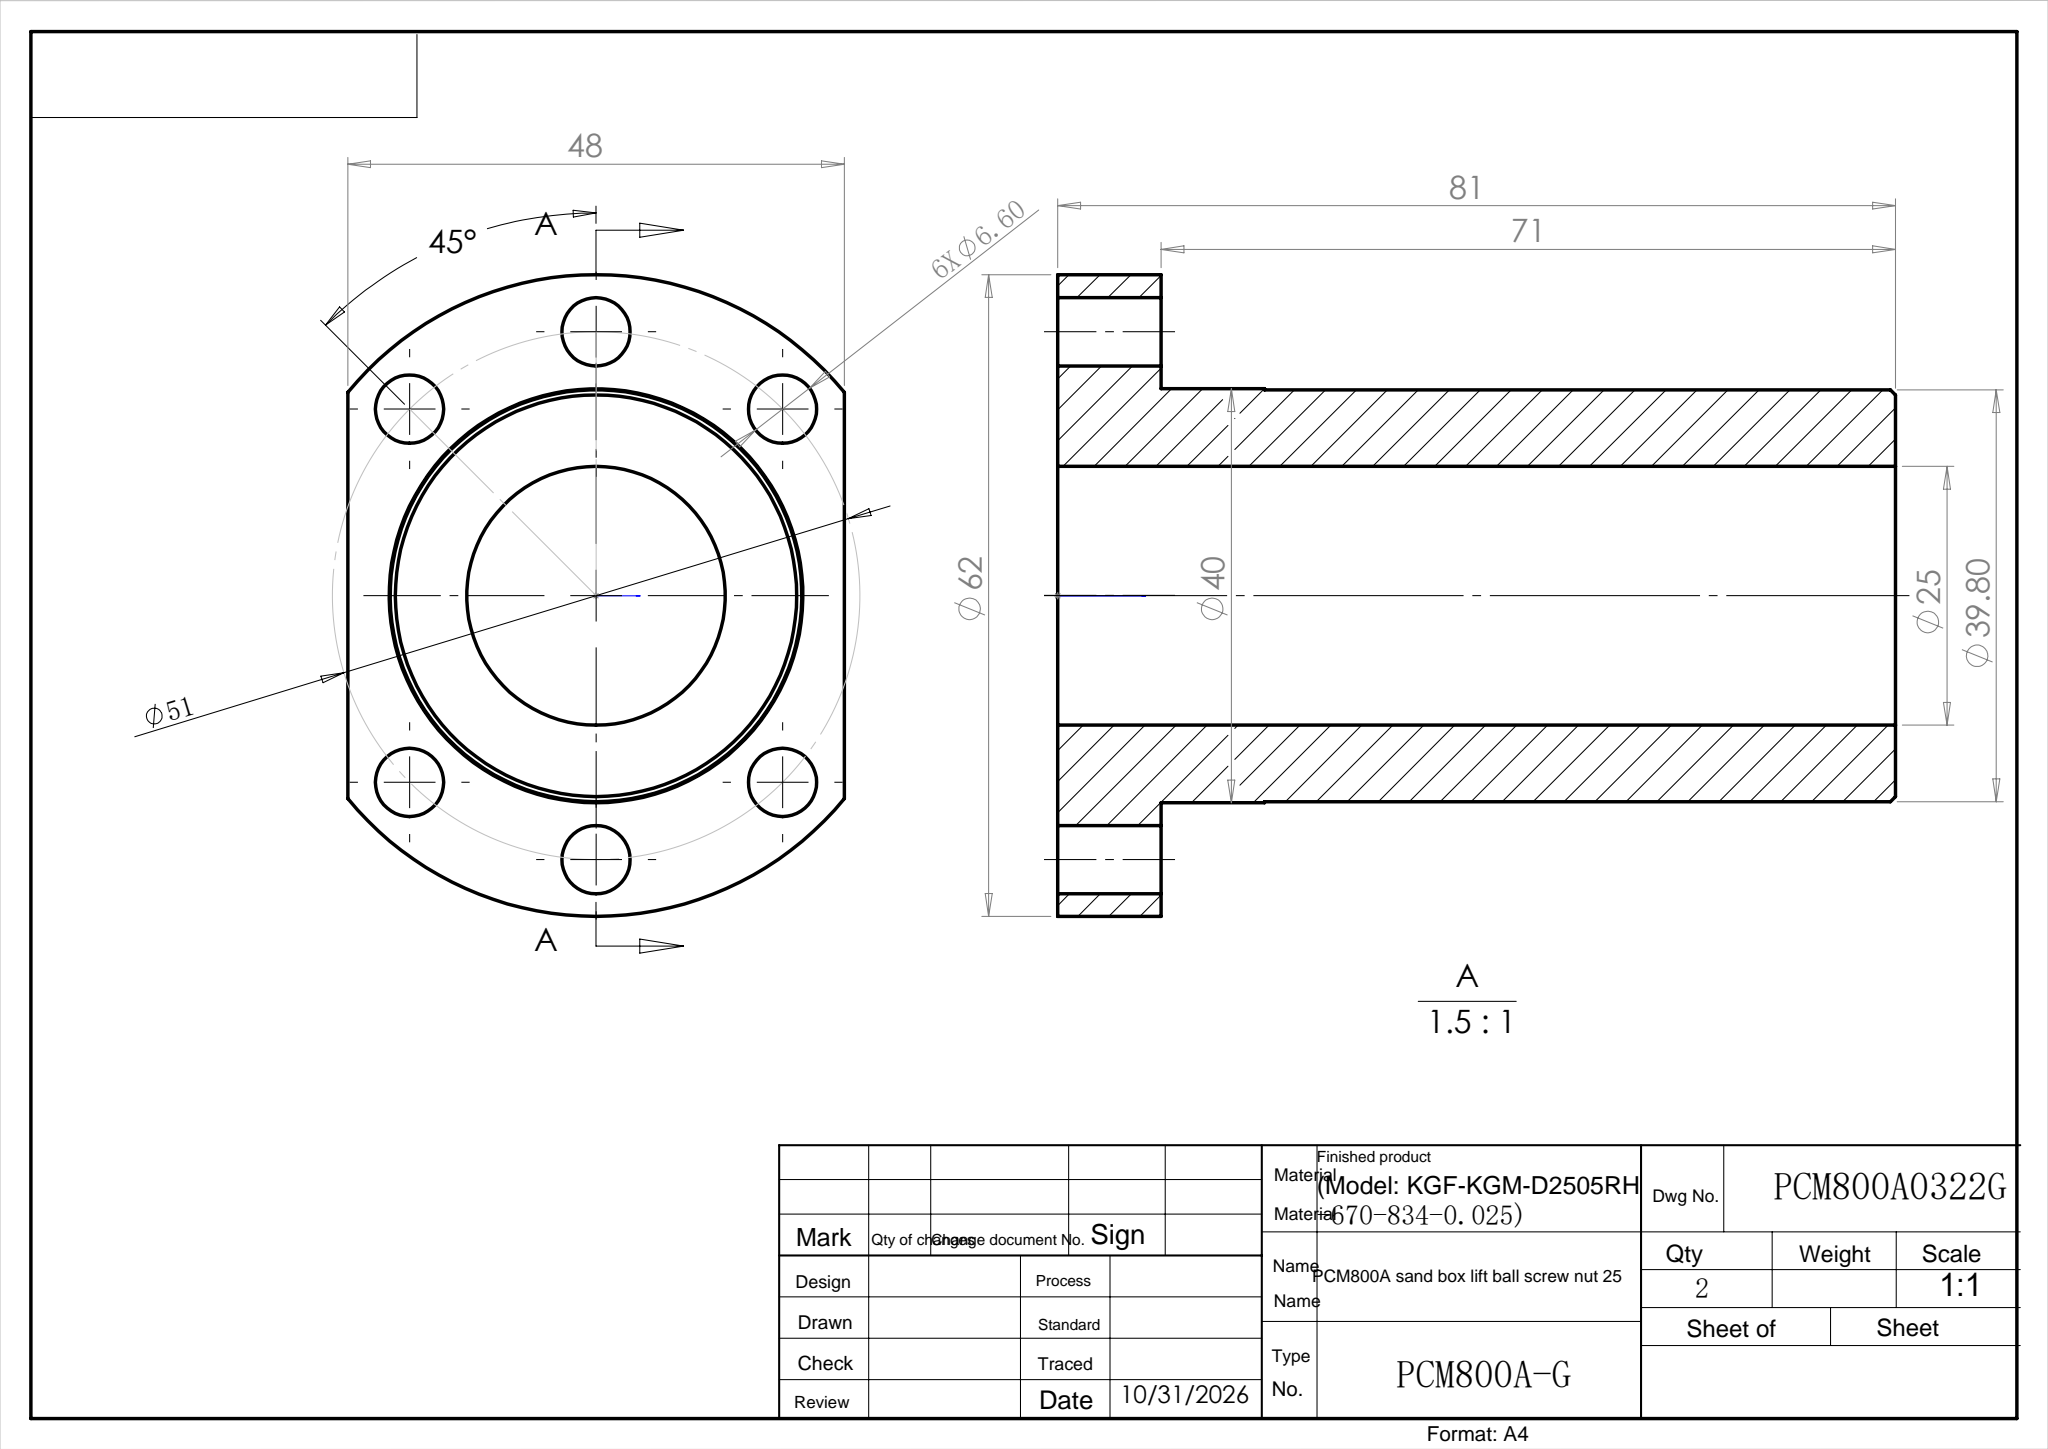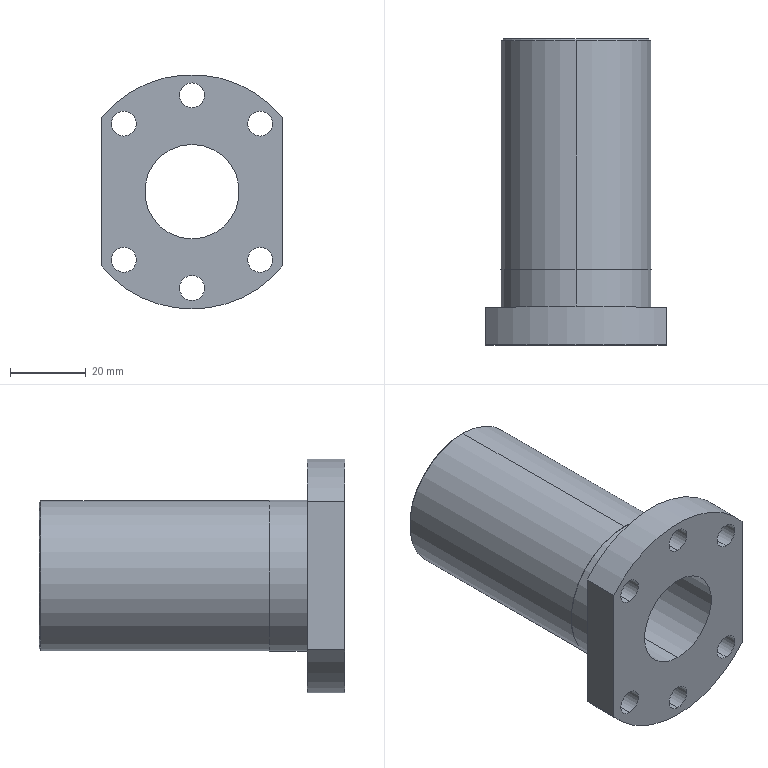Part | SolidWorks | features Boss 2, Cut 2, Chamfer 1, Extrusion 1 | 1 solid | 29 faces | box 48 x 81 x 62 mm | volume 73064 mm3 | cylinder 21 | plane 6 | cone 2 | commonest cylinder face diameters 6.6 x12 62 x3 25 x2 39.8 x2 40 x2
STEP:
#1=CARTESIAN_POINT('',(0.,81.,19.4));
#2=VERTEX_POINT('',#1);
#3=CARTESIAN_POINT('',(0.,81.,-19.4));
#4=VERTEX_POINT('',#3);
#5=CARTESIAN_POINT('',(0.,81.,0.));
#6=DIRECTION('',(0.,1.,0.));
#7=DIRECTION('',(0.,0.,1.));
#8=AXIS2_PLACEMENT_3D('',#5,#6,#7);
#9=CIRCLE('',#8,19.4);
#10=EDGE_CURVE('',#2,#4,#9,.T.);
#11=ORIENTED_EDGE('',*,*,#10,.F.);
#12=CARTESIAN_POINT('',(0.,80.5,19.9));
#13=VERTEX_POINT('',#12);
#14=CARTESIAN_POINT('',(0.,81.,19.4));
#15=DIRECTION('',(0.,-0.7071,0.7071));
#16=VECTOR('',#15,1000.);
#17=LINE('',#14,#16);
#18=EDGE_CURVE('',#2,#13,#17,.T.);
#19=ORIENTED_EDGE('',*,*,#18,.T.);
#20=CARTESIAN_POINT('',(0.,80.5,-19.9));
#21=VERTEX_POINT('',#20);
#22=CARTESIAN_POINT('',(0.,80.5,0.));
#23=DIRECTION('',(0.,-1.,0.));
#24=DIRECTION('',(0.,0.,1.));
#25=AXIS2_PLACEMENT_3D('',#22,#23,#24);
#26=CIRCLE('',#25,19.9);
#27=EDGE_CURVE('',#21,#13,#26,.T.);
#28=ORIENTED_EDGE('',*,*,#27,.F.);
#29=CARTESIAN_POINT('',(0.,81.,-19.4));
#30=DIRECTION('',(0.,-0.7071,-0.7071));
#31=VECTOR('',#30,1000.);
#32=LINE('',#29,#31);
#33=EDGE_CURVE('',#4,#21,#32,.T.);
#34=ORIENTED_EDGE('',*,*,#33,.F.);
#35=EDGE_LOOP('',(#11,#19,#28,#34));
#36=FACE_OUTER_BOUND('',#35,.T.);
#37=CARTESIAN_POINT('',(0.,81.,0.));
#38=DIRECTION('',(0.,-1.,0.));
#39=DIRECTION('',(0.,0.,-1.));
#40=AXIS2_PLACEMENT_3D('',#37,#38,#39);
#41=CONICAL_SURFACE('',#40,19.4,0.7854);
#42=ADVANCED_FACE('',(#36),#41,.T.);
#43=CARTESIAN_POINT('',(18.031,10.,14.731));
#44=VERTEX_POINT('',#43);
#45=CARTESIAN_POINT('',(18.031,10.,21.331));
#46=VERTEX_POINT('',#45);
#47=CARTESIAN_POINT('',(18.031,10.,18.031));
#48=DIRECTION('',(0.,1.,0.));
#49=DIRECTION('',(0.,0.,1.));
#50=AXIS2_PLACEMENT_3D('',#47,#48,#49);
#51=CIRCLE('',#50,3.3);
#52=EDGE_CURVE('',#44,#46,#51,.T.);
#53=ORIENTED_EDGE('',*,*,#52,.T.);
#54=CARTESIAN_POINT('',(18.031,0.,21.331));
#55=VERTEX_POINT('',#54);
#56=CARTESIAN_POINT('',(18.031,81.,21.331));
#57=DIRECTION('',(0.,-1.,0.));
#58=VECTOR('',#57,1000.);
#59=LINE('',#56,#58);
#60=EDGE_CURVE('',#46,#55,#59,.T.);
#61=ORIENTED_EDGE('',*,*,#60,.T.);
#62=CARTESIAN_POINT('',(18.031,0.,14.731));
#63=VERTEX_POINT('',#62);
#64=CARTESIAN_POINT('',(18.031,0.,18.031));
#65=DIRECTION('',(0.,-1.,0.));
#66=DIRECTION('',(0.,0.,-1.));
#67=AXIS2_PLACEMENT_3D('',#64,#65,#66);
#68=CIRCLE('',#67,3.3);
#69=EDGE_CURVE('',#55,#63,#68,.T.);
#70=ORIENTED_EDGE('',*,*,#69,.T.);
#71=CARTESIAN_POINT('',(18.031,81.,14.731));
#72=DIRECTION('',(0.,-1.,0.));
#73=VECTOR('',#72,1000.);
#74=LINE('',#71,#73);
#75=EDGE_CURVE('',#44,#63,#74,.T.);
#76=ORIENTED_EDGE('',*,*,#75,.F.);
#77=EDGE_LOOP('',(#53,#61,#70,#76));
#78=FACE_OUTER_BOUND('',#77,.T.);
#79=CARTESIAN_POINT('',(18.031,81.,18.031));
#80=DIRECTION('',(0.,-1.,0.));
#81=DIRECTION('',(0.,0.,-1.));
#82=AXIS2_PLACEMENT_3D('',#79,#80,#81);
#83=CYLINDRICAL_SURFACE('',#82,3.3);
#84=ADVANCED_FACE('',(#78),#83,.F.);
#85=CARTESIAN_POINT('',(0.,10.,22.2));
#86=VERTEX_POINT('',#85);
#87=CARTESIAN_POINT('',(0.,10.,28.8));
#88=VERTEX_POINT('',#87);
#89=CARTESIAN_POINT('',(0.,10.,25.5));
#90=DIRECTION('',(0.,1.,0.));
#91=DIRECTION('',(0.,0.,1.));
#92=AXIS2_PLACEMENT_3D('',#89,#90,#91);
#93=CIRCLE('',#92,3.3);
#94=EDGE_CURVE('',#86,#88,#93,.T.);
#95=ORIENTED_EDGE('',*,*,#94,.T.);
#96=CARTESIAN_POINT('',(0.,0.,28.8));
#97=VERTEX_POINT('',#96);
#98=CARTESIAN_POINT('',(0.,81.,28.8));
#99=DIRECTION('',(0.,-1.,0.));
#100=VECTOR('',#99,1000.);
#101=LINE('',#98,#100);
#102=EDGE_CURVE('',#88,#97,#101,.T.);
#103=ORIENTED_EDGE('',*,*,#102,.T.);
#104=CARTESIAN_POINT('',(0.,0.,22.2));
#105=VERTEX_POINT('',#104);
#106=CARTESIAN_POINT('',(0.,0.,25.5));
#107=DIRECTION('',(0.,-1.,0.));
#108=DIRECTION('',(0.,0.,-1.));
#109=AXIS2_PLACEMENT_3D('',#106,#107,#108);
#110=CIRCLE('',#109,3.3);
#111=EDGE_CURVE('',#97,#105,#110,.T.);
#112=ORIENTED_EDGE('',*,*,#111,.T.);
#113=CARTESIAN_POINT('',(0.,81.,22.2));
#114=DIRECTION('',(0.,-1.,0.));
#115=VECTOR('',#114,1000.);
#116=LINE('',#113,#115);
#117=EDGE_CURVE('',#86,#105,#116,.T.);
#118=ORIENTED_EDGE('',*,*,#117,.F.);
#119=EDGE_LOOP('',(#95,#103,#112,#118));
#120=FACE_OUTER_BOUND('',#119,.T.);
#121=CARTESIAN_POINT('',(0.,81.,25.5));
#122=DIRECTION('',(0.,-1.,0.));
#123=DIRECTION('',(0.,0.,-1.));
#124=AXIS2_PLACEMENT_3D('',#121,#122,#123);
#125=CYLINDRICAL_SURFACE('',#124,3.3);
#126=ADVANCED_FACE('',(#120),#125,.F.);
#127=CARTESIAN_POINT('',(-18.031,10.,14.731));
#128=VERTEX_POINT('',#127);
#129=CARTESIAN_POINT('',(-18.031,10.,21.331));
#130=VERTEX_POINT('',#129);
#131=CARTESIAN_POINT('',(-18.031,10.,18.031));
#132=DIRECTION('',(0.,1.,0.));
#133=DIRECTION('',(0.,0.,1.));
#134=AXIS2_PLACEMENT_3D('',#131,#132,#133);
#135=CIRCLE('',#134,3.3);
#136=EDGE_CURVE('',#128,#130,#135,.T.);
#137=ORIENTED_EDGE('',*,*,#136,.T.);
#138=CARTESIAN_POINT('',(-18.031,0.,21.331));
#139=VERTEX_POINT('',#138);
#140=CARTESIAN_POINT('',(-18.031,81.,21.331));
#141=DIRECTION('',(0.,-1.,0.));
#142=VECTOR('',#141,1000.);
#143=LINE('',#140,#142);
#144=EDGE_CURVE('',#130,#139,#143,.T.);
#145=ORIENTED_EDGE('',*,*,#144,.T.);
#146=CARTESIAN_POINT('',(-18.031,0.,14.731));
#147=VERTEX_POINT('',#146);
#148=CARTESIAN_POINT('',(-18.031,0.,18.031));
#149=DIRECTION('',(0.,-1.,0.));
#150=DIRECTION('',(0.,0.,-1.));
#151=AXIS2_PLACEMENT_3D('',#148,#149,#150);
#152=CIRCLE('',#151,3.3);
#153=EDGE_CURVE('',#139,#147,#152,.T.);
#154=ORIENTED_EDGE('',*,*,#153,.T.);
#155=CARTESIAN_POINT('',(-18.031,81.,14.731));
#156=DIRECTION('',(0.,-1.,0.));
#157=VECTOR('',#156,1000.);
#158=LINE('',#155,#157);
#159=EDGE_CURVE('',#128,#147,#158,.T.);
#160=ORIENTED_EDGE('',*,*,#159,.F.);
#161=EDGE_LOOP('',(#137,#145,#154,#160));
#162=FACE_OUTER_BOUND('',#161,.T.);
#163=CARTESIAN_POINT('',(-18.031,81.,18.031));
#164=DIRECTION('',(0.,-1.,0.));
#165=DIRECTION('',(0.,0.,-1.));
#166=AXIS2_PLACEMENT_3D('',#163,#164,#165);
#167=CYLINDRICAL_SURFACE('',#166,3.3);
#168=ADVANCED_FACE('',(#162),#167,.F.);
#169=CARTESIAN_POINT('',(-18.031,10.,-21.331));
#170=VERTEX_POINT('',#169);
#171=CARTESIAN_POINT('',(-18.031,10.,-14.731));
#172=VERTEX_POINT('',#171);
#173=CARTESIAN_POINT('',(-18.031,10.,-18.031));
#174=DIRECTION('',(0.,1.,0.));
#175=DIRECTION('',(0.,0.,1.));
#176=AXIS2_PLACEMENT_3D('',#173,#174,#175);
#177=CIRCLE('',#176,3.3);
#178=EDGE_CURVE('',#170,#172,#177,.T.);
#179=ORIENTED_EDGE('',*,*,#178,.T.);
#180=CARTESIAN_POINT('',(-18.031,0.,-14.731));
#181=VERTEX_POINT('',#180);
#182=CARTESIAN_POINT('',(-18.031,81.,-14.731));
#183=DIRECTION('',(0.,-1.,0.));
#184=VECTOR('',#183,1000.);
#185=LINE('',#182,#184);
#186=EDGE_CURVE('',#172,#181,#185,.T.);
#187=ORIENTED_EDGE('',*,*,#186,.T.);
#188=CARTESIAN_POINT('',(-18.031,0.,-21.331));
#189=VERTEX_POINT('',#188);
#190=CARTESIAN_POINT('',(-18.031,0.,-18.031));
#191=DIRECTION('',(0.,-1.,0.));
#192=DIRECTION('',(0.,0.,-1.));
#193=AXIS2_PLACEMENT_3D('',#190,#191,#192);
#194=CIRCLE('',#193,3.3);
#195=EDGE_CURVE('',#181,#189,#194,.T.);
#196=ORIENTED_EDGE('',*,*,#195,.T.);
#197=CARTESIAN_POINT('',(-18.031,81.,-21.331));
#198=DIRECTION('',(0.,-1.,0.));
#199=VECTOR('',#198,1000.);
#200=LINE('',#197,#199);
#201=EDGE_CURVE('',#170,#189,#200,.T.);
#202=ORIENTED_EDGE('',*,*,#201,.F.);
#203=EDGE_LOOP('',(#179,#187,#196,#202));
#204=FACE_OUTER_BOUND('',#203,.T.);
#205=CARTESIAN_POINT('',(-18.031,81.,-18.031));
#206=DIRECTION('',(0.,-1.,0.));
#207=DIRECTION('',(0.,0.,-1.));
#208=AXIS2_PLACEMENT_3D('',#205,#206,#207);
#209=CYLINDRICAL_SURFACE('',#208,3.3);
#210=ADVANCED_FACE('',(#204),#209,.F.);
#211=CARTESIAN_POINT('',(0.,10.,-28.8));
#212=VERTEX_POINT('',#211);
#213=CARTESIAN_POINT('',(0.,10.,-22.2));
#214=VERTEX_POINT('',#213);
#215=CARTESIAN_POINT('',(0.,10.,-25.5));
#216=DIRECTION('',(0.,1.,0.));
#217=DIRECTION('',(0.,0.,1.));
#218=AXIS2_PLACEMENT_3D('',#215,#216,#217);
#219=CIRCLE('',#218,3.3);
#220=EDGE_CURVE('',#212,#214,#219,.T.);
#221=ORIENTED_EDGE('',*,*,#220,.T.);
#222=CARTESIAN_POINT('',(0.,0.,-22.2));
#223=VERTEX_POINT('',#222);
#224=CARTESIAN_POINT('',(0.,81.,-22.2));
#225=DIRECTION('',(0.,-1.,0.));
#226=VECTOR('',#225,1000.);
#227=LINE('',#224,#226);
#228=EDGE_CURVE('',#214,#223,#227,.T.);
#229=ORIENTED_EDGE('',*,*,#228,.T.);
#230=CARTESIAN_POINT('',(0.,0.,-28.8));
#231=VERTEX_POINT('',#230);
#232=CARTESIAN_POINT('',(0.,0.,-25.5));
#233=DIRECTION('',(0.,-1.,0.));
#234=DIRECTION('',(0.,0.,-1.));
#235=AXIS2_PLACEMENT_3D('',#232,#233,#234);
#236=CIRCLE('',#235,3.3);
#237=EDGE_CURVE('',#223,#231,#236,.T.);
#238=ORIENTED_EDGE('',*,*,#237,.T.);
#239=CARTESIAN_POINT('',(0.,81.,-28.8));
#240=DIRECTION('',(0.,-1.,0.));
#241=VECTOR('',#240,1000.);
#242=LINE('',#239,#241);
#243=EDGE_CURVE('',#212,#231,#242,.T.);
#244=ORIENTED_EDGE('',*,*,#243,.F.);
#245=EDGE_LOOP('',(#221,#229,#238,#244));
#246=FACE_OUTER_BOUND('',#245,.T.);
#247=CARTESIAN_POINT('',(0.,81.,-25.5));
#248=DIRECTION('',(0.,-1.,0.));
#249=DIRECTION('',(0.,0.,-1.));
#250=AXIS2_PLACEMENT_3D('',#247,#248,#249);
#251=CYLINDRICAL_SURFACE('',#250,3.3);
#252=ADVANCED_FACE('',(#246),#251,.F.);
#253=CARTESIAN_POINT('',(18.031,10.,-21.331));
#254=VERTEX_POINT('',#253);
#255=CARTESIAN_POINT('',(18.031,10.,-14.731));
#256=VERTEX_POINT('',#255);
#257=CARTESIAN_POINT('',(18.031,10.,-18.031));
#258=DIRECTION('',(0.,1.,0.));
#259=DIRECTION('',(0.,0.,1.));
#260=AXIS2_PLACEMENT_3D('',#257,#258,#259);
#261=CIRCLE('',#260,3.3);
#262=EDGE_CURVE('',#254,#256,#261,.T.);
#263=ORIENTED_EDGE('',*,*,#262,.T.);
#264=CARTESIAN_POINT('',(18.031,0.,-14.731));
#265=VERTEX_POINT('',#264);
#266=CARTESIAN_POINT('',(18.031,81.,-14.731));
#267=DIRECTION('',(0.,-1.,0.));
#268=VECTOR('',#267,1000.);
#269=LINE('',#266,#268);
#270=EDGE_CURVE('',#256,#265,#269,.T.);
#271=ORIENTED_EDGE('',*,*,#270,.T.);
#272=CARTESIAN_POINT('',(18.031,0.,-21.331));
#273=VERTEX_POINT('',#272);
#274=CARTESIAN_POINT('',(18.031,0.,-18.031));
#275=DIRECTION('',(0.,-1.,0.));
#276=DIRECTION('',(0.,0.,-1.));
#277=AXIS2_PLACEMENT_3D('',#274,#275,#276);
#278=CIRCLE('',#277,3.3);
#279=EDGE_CURVE('',#265,#273,#278,.T.);
#280=ORIENTED_EDGE('',*,*,#279,.T.);
#281=CARTESIAN_POINT('',(18.031,81.,-21.331));
#282=DIRECTION('',(0.,-1.,0.));
#283=VECTOR('',#282,1000.);
#284=LINE('',#281,#283);
#285=EDGE_CURVE('',#254,#273,#284,.T.);
#286=ORIENTED_EDGE('',*,*,#285,.F.);
#287=EDGE_LOOP('',(#263,#271,#280,#286));
#288=FACE_OUTER_BOUND('',#287,.T.);
#289=CARTESIAN_POINT('',(18.031,81.,-18.031));
#290=DIRECTION('',(0.,-1.,0.));
#291=DIRECTION('',(0.,0.,-1.));
#292=AXIS2_PLACEMENT_3D('',#289,#290,#291);
#293=CYLINDRICAL_SURFACE('',#292,3.3);
#294=ADVANCED_FACE('',(#288),#293,.F.);
#295=CARTESIAN_POINT('',(0.,0.,-12.5));
#296=VERTEX_POINT('',#295);
#297=CARTESIAN_POINT('',(0.,0.,12.5));
#298=VERTEX_POINT('',#297);
#299=CARTESIAN_POINT('',(0.,0.,0.));
#300=DIRECTION('',(0.,1.,0.));
#301=DIRECTION('',(0.,0.,1.));
#302=AXIS2_PLACEMENT_3D('',#299,#300,#301);
#303=CIRCLE('',#302,12.5);
#304=EDGE_CURVE('',#296,#298,#303,.T.);
#305=ORIENTED_EDGE('',*,*,#304,.F.);
#306=CARTESIAN_POINT('',(0.,81.,-12.5));
#307=VERTEX_POINT('',#306);
#308=CARTESIAN_POINT('',(0.,0.,-12.5));
#309=DIRECTION('',(0.,1.,0.));
#310=VECTOR('',#309,1000.);
#311=LINE('',#308,#310);
#312=EDGE_CURVE('',#296,#307,#311,.T.);
#313=ORIENTED_EDGE('',*,*,#312,.T.);
#314=CARTESIAN_POINT('',(0.,81.,12.5));
#315=VERTEX_POINT('',#314);
#316=CARTESIAN_POINT('',(0.,81.,0.));
#317=DIRECTION('',(0.,1.,0.));
#318=DIRECTION('',(0.,0.,1.));
#319=AXIS2_PLACEMENT_3D('',#316,#317,#318);
#320=CIRCLE('',#319,12.5);
#321=EDGE_CURVE('',#307,#315,#320,.T.);
#322=ORIENTED_EDGE('',*,*,#321,.T.);
#323=CARTESIAN_POINT('',(0.,0.,12.5));
#324=DIRECTION('',(0.,1.,0.));
#325=VECTOR('',#324,1000.);
#326=LINE('',#323,#325);
#327=EDGE_CURVE('',#298,#315,#326,.T.);
#328=ORIENTED_EDGE('',*,*,#327,.F.);
#329=EDGE_LOOP('',(#305,#313,#322,#328));
#330=FACE_OUTER_BOUND('',#329,.T.);
#331=CARTESIAN_POINT('',(0.,0.,0.));
#332=DIRECTION('',(0.,1.,0.));
#333=DIRECTION('',(0.,0.,1.));
#334=AXIS2_PLACEMENT_3D('',#331,#332,#333);
#335=CYLINDRICAL_SURFACE('',#334,12.5);
#336=ADVANCED_FACE('',(#330),#335,.F.);
#337=ORIENTED_EDGE('',*,*,#27,.T.);
#338=CARTESIAN_POINT('',(0.,20.,19.9));
#339=VERTEX_POINT('',#338);
#340=CARTESIAN_POINT('',(0.,81.,19.9));
#341=DIRECTION('',(0.,-1.,0.));
#342=VECTOR('',#341,1000.);
#343=LINE('',#340,#342);
#344=EDGE_CURVE('',#13,#339,#343,.T.);
#345=ORIENTED_EDGE('',*,*,#344,.T.);
#346=CARTESIAN_POINT('',(0.,20.,-19.9));
#347=VERTEX_POINT('',#346);
#348=CARTESIAN_POINT('',(0.,20.,0.));
#349=DIRECTION('',(0.,1.,0.));
#350=DIRECTION('',(0.,0.,1.));
#351=AXIS2_PLACEMENT_3D('',#348,#349,#350);
#352=CIRCLE('',#351,19.9);
#353=EDGE_CURVE('',#339,#347,#352,.T.);
#354=ORIENTED_EDGE('',*,*,#353,.T.);
#355=CARTESIAN_POINT('',(0.,81.,-19.9));
#356=DIRECTION('',(0.,-1.,0.));
#357=VECTOR('',#356,1000.);
#358=LINE('',#355,#357);
#359=EDGE_CURVE('',#21,#347,#358,.T.);
#360=ORIENTED_EDGE('',*,*,#359,.F.);
#361=EDGE_LOOP('',(#337,#345,#354,#360));
#362=FACE_OUTER_BOUND('',#361,.T.);
#363=CARTESIAN_POINT('',(0.,81.,0.));
#364=DIRECTION('',(0.,-1.,0.));
#365=DIRECTION('',(0.,0.,-1.));
#366=AXIS2_PLACEMENT_3D('',#363,#364,#365);
#367=CYLINDRICAL_SURFACE('',#366,19.9);
#368=ADVANCED_FACE('',(#362),#367,.T.);
#369=CARTESIAN_POINT('',(0.,20.,20.));
#370=VERTEX_POINT('',#369);
#371=CARTESIAN_POINT('',(0.,20.,-20.));
#372=VERTEX_POINT('',#371);
#373=CARTESIAN_POINT('',(0.,20.,0.));
#374=DIRECTION('',(0.,1.,0.));
#375=DIRECTION('',(0.,0.,1.));
#376=AXIS2_PLACEMENT_3D('',#373,#374,#375);
#377=CIRCLE('',#376,20.);
#378=EDGE_CURVE('',#370,#372,#377,.T.);
#379=ORIENTED_EDGE('',*,*,#378,.F.);
#380=CARTESIAN_POINT('',(0.,10.,20.));
#381=VERTEX_POINT('',#380);
#382=CARTESIAN_POINT('',(0.,20.,20.));
#383=DIRECTION('',(0.,-1.,0.));
#384=VECTOR('',#383,1000.);
#385=LINE('',#382,#384);
#386=EDGE_CURVE('',#370,#381,#385,.T.);
#387=ORIENTED_EDGE('',*,*,#386,.T.);
#388=CARTESIAN_POINT('',(0.,10.,-20.));
#389=VERTEX_POINT('',#388);
#390=CARTESIAN_POINT('',(0.,10.,0.));
#391=DIRECTION('',(0.,1.,0.));
#392=DIRECTION('',(0.,0.,1.));
#393=AXIS2_PLACEMENT_3D('',#390,#391,#392);
#394=CIRCLE('',#393,20.);
#395=EDGE_CURVE('',#381,#389,#394,.T.);
#396=ORIENTED_EDGE('',*,*,#395,.T.);
#397=CARTESIAN_POINT('',(0.,20.,-20.));
#398=DIRECTION('',(0.,-1.,0.));
#399=VECTOR('',#398,1000.);
#400=LINE('',#397,#399);
#401=EDGE_CURVE('',#372,#389,#400,.T.);
#402=ORIENTED_EDGE('',*,*,#401,.F.);
#403=EDGE_LOOP('',(#379,#387,#396,#402));
#404=FACE_OUTER_BOUND('',#403,.T.);
#405=CARTESIAN_POINT('',(0.,20.,0.));
#406=DIRECTION('',(0.,-1.,0.));
#407=DIRECTION('',(0.,0.,-1.));
#408=AXIS2_PLACEMENT_3D('',#405,#406,#407);
#409=CYLINDRICAL_SURFACE('',#408,20.);
#410=ADVANCED_FACE('',(#404),#409,.T.);
#411=CARTESIAN_POINT('',(0.,10.,-31.026));
#412=VERTEX_POINT('',#411);
#413=CARTESIAN_POINT('',(-24.,10.,-19.647));
#414=VERTEX_POINT('',#413);
#415=CARTESIAN_POINT('',(0.,10.,-0.02605));
#416=DIRECTION('',(0.,1.,0.));
#417=DIRECTION('',(0.,0.,1.));
#418=AXIS2_PLACEMENT_3D('',#415,#416,#417);
#419=CIRCLE('',#418,31.);
#420=EDGE_CURVE('',#412,#414,#419,.T.);
#421=ORIENTED_EDGE('',*,*,#420,.F.);
#422=CARTESIAN_POINT('',(0.,0.,-31.026));
#423=VERTEX_POINT('',#422);
#424=CARTESIAN_POINT('',(0.,10.,-31.026));
#425=DIRECTION('',(0.,-1.,0.));
#426=VECTOR('',#425,1000.);
#427=LINE('',#424,#426);
#428=EDGE_CURVE('',#412,#423,#427,.T.);
#429=ORIENTED_EDGE('',*,*,#428,.T.);
#430=CARTESIAN_POINT('',(-24.,0.,-19.647));
#431=VERTEX_POINT('',#430);
#432=CARTESIAN_POINT('',(0.,0.,-0.02605));
#433=DIRECTION('',(0.,1.,0.));
#434=DIRECTION('',(0.,0.,1.));
#435=AXIS2_PLACEMENT_3D('',#432,#433,#434);
#436=CIRCLE('',#435,31.);
#437=EDGE_CURVE('',#423,#431,#436,.T.);
#438=ORIENTED_EDGE('',*,*,#437,.T.);
#439=CARTESIAN_POINT('',(-24.,10.,-19.647));
#440=DIRECTION('',(0.,-1.,0.));
#441=VECTOR('',#440,1000.);
#442=LINE('',#439,#441);
#443=EDGE_CURVE('',#414,#431,#442,.T.);
#444=ORIENTED_EDGE('',*,*,#443,.F.);
#445=EDGE_LOOP('',(#421,#429,#438,#444));
#446=FACE_OUTER_BOUND('',#445,.T.);
#447=CARTESIAN_POINT('',(0.,10.,-0.02605));
#448=DIRECTION('',(0.,-1.,0.));
#449=DIRECTION('',(0.,0.,-1.));
#450=AXIS2_PLACEMENT_3D('',#447,#448,#449);
#451=CYLINDRICAL_SURFACE('',#450,31.);
#452=ADVANCED_FACE('',(#446),#451,.T.);
#453=CARTESIAN_POINT('',(0.,20.,0.));
#454=DIRECTION('',(0.,1.,0.));
#455=DIRECTION('',(0.,0.,1.));
#456=AXIS2_PLACEMENT_3D('',#453,#454,#455);
#457=CIRCLE('',#456,20.);
#458=EDGE_CURVE('',#372,#370,#457,.T.);
#459=ORIENTED_EDGE('',*,*,#458,.T.);
#460=ORIENTED_EDGE('',*,*,#378,.T.);
#461=EDGE_LOOP('',(#459,#460));
#462=FACE_OUTER_BOUND('',#461,.T.);
#463=CARTESIAN_POINT('',(0.,20.,0.));
#464=DIRECTION('',(0.,1.,0.));
#465=DIRECTION('',(0.,0.,1.));
#466=AXIS2_PLACEMENT_3D('',#463,#464,#465);
#467=CIRCLE('',#466,19.9);
#468=EDGE_CURVE('',#347,#339,#467,.T.);
#469=ORIENTED_EDGE('',*,*,#468,.F.);
#470=ORIENTED_EDGE('',*,*,#353,.F.);
#471=EDGE_LOOP('',(#469,#470));
#472=FACE_BOUND('',#471,.T.);
#473=CARTESIAN_POINT('',(0.,20.,0.));
#474=DIRECTION('',(0.,1.,0.));
#475=DIRECTION('',(0.,0.,1.));
#476=AXIS2_PLACEMENT_3D('',#473,#474,#475);
#477=PLANE('',#476);
#478=ADVANCED_FACE('',(#462,#472),#477,.T.);
#479=ORIENTED_EDGE('',*,*,#52,.F.);
#480=CARTESIAN_POINT('',(18.031,10.,18.031));
#481=DIRECTION('',(0.,1.,0.));
#482=DIRECTION('',(0.,0.,1.));
#483=AXIS2_PLACEMENT_3D('',#480,#481,#482);
#484=CIRCLE('',#483,3.3);
#485=EDGE_CURVE('',#46,#44,#484,.T.);
#486=ORIENTED_EDGE('',*,*,#485,.F.);
#487=EDGE_LOOP('',(#479,#486));
#488=FACE_BOUND('',#487,.T.);
#489=ORIENTED_EDGE('',*,*,#94,.F.);
#490=CARTESIAN_POINT('',(0.,10.,25.5));
#491=DIRECTION('',(0.,1.,0.));
#492=DIRECTION('',(0.,0.,1.));
#493=AXIS2_PLACEMENT_3D('',#490,#491,#492);
#494=CIRCLE('',#493,3.3);
#495=EDGE_CURVE('',#88,#86,#494,.T.);
#496=ORIENTED_EDGE('',*,*,#495,.F.);
#497=EDGE_LOOP('',(#489,#496));
#498=FACE_BOUND('',#497,.T.);
#499=ORIENTED_EDGE('',*,*,#136,.F.);
#500=CARTESIAN_POINT('',(-18.031,10.,18.031));
#501=DIRECTION('',(0.,1.,0.));
#502=DIRECTION('',(0.,0.,1.));
#503=AXIS2_PLACEMENT_3D('',#500,#501,#502);
#504=CIRCLE('',#503,3.3);
#505=EDGE_CURVE('',#130,#128,#504,.T.);
#506=ORIENTED_EDGE('',*,*,#505,.F.);
#507=EDGE_LOOP('',(#499,#506));
#508=FACE_BOUND('',#507,.T.);
#509=ORIENTED_EDGE('',*,*,#178,.F.);
#510=CARTESIAN_POINT('',(-18.031,10.,-18.031));
#511=DIRECTION('',(0.,1.,0.));
#512=DIRECTION('',(0.,0.,1.));
#513=AXIS2_PLACEMENT_3D('',#510,#511,#512);
#514=CIRCLE('',#513,3.3);
#515=EDGE_CURVE('',#172,#170,#514,.T.);
#516=ORIENTED_EDGE('',*,*,#515,.F.);
#517=EDGE_LOOP('',(#509,#516));
#518=FACE_BOUND('',#517,.T.);
#519=ORIENTED_EDGE('',*,*,#220,.F.);
#520=CARTESIAN_POINT('',(0.,10.,-25.5));
#521=DIRECTION('',(0.,1.,0.));
#522=DIRECTION('',(0.,0.,1.));
#523=AXIS2_PLACEMENT_3D('',#520,#521,#522);
#524=CIRCLE('',#523,3.3);
#525=EDGE_CURVE('',#214,#212,#524,.T.);
#526=ORIENTED_EDGE('',*,*,#525,.F.);
#527=EDGE_LOOP('',(#519,#526));
#528=FACE_BOUND('',#527,.T.);
#529=ORIENTED_EDGE('',*,*,#262,.F.);
#530=CARTESIAN_POINT('',(18.031,10.,-18.031));
#531=DIRECTION('',(0.,1.,0.));
#532=DIRECTION('',(0.,0.,1.));
#533=AXIS2_PLACEMENT_3D('',#530,#531,#532);
#534=CIRCLE('',#533,3.3);
#535=EDGE_CURVE('',#256,#254,#534,.T.);
#536=ORIENTED_EDGE('',*,*,#535,.F.);
#537=EDGE_LOOP('',(#529,#536));
#538=FACE_BOUND('',#537,.T.);
#539=CARTESIAN_POINT('',(-24.,10.,19.595));
#540=VERTEX_POINT('',#539);
#541=CARTESIAN_POINT('',(24.,10.,19.595));
#542=VERTEX_POINT('',#541);
#543=CARTESIAN_POINT('',(0.,10.,-0.02605));
#544=DIRECTION('',(0.,1.,0.));
#545=DIRECTION('',(0.,0.,1.));
#546=AXIS2_PLACEMENT_3D('',#543,#544,#545);
#547=CIRCLE('',#546,31.);
#548=EDGE_CURVE('',#540,#542,#547,.T.);
#549=ORIENTED_EDGE('',*,*,#548,.T.);
#550=CARTESIAN_POINT('',(24.,10.,-19.647));
#551=VERTEX_POINT('',#550);
#552=CARTESIAN_POINT('',(24.,10.,19.595));
#553=DIRECTION('',(0.,0.,-1.));
#554=VECTOR('',#553,1000.);
#555=LINE('',#552,#554);
#556=EDGE_CURVE('',#542,#551,#555,.T.);
#557=ORIENTED_EDGE('',*,*,#556,.T.);
#558=CARTESIAN_POINT('',(0.,10.,-0.02605));
#559=DIRECTION('',(0.,1.,0.));
#560=DIRECTION('',(0.,0.,1.));
#561=AXIS2_PLACEMENT_3D('',#558,#559,#560);
#562=CIRCLE('',#561,31.);
#563=EDGE_CURVE('',#551,#412,#562,.T.);
#564=ORIENTED_EDGE('',*,*,#563,.T.);
#565=ORIENTED_EDGE('',*,*,#420,.T.);
#566=CARTESIAN_POINT('',(-24.,10.,19.595));
#567=DIRECTION('',(0.,0.,1.));
#568=VECTOR('',#567,1000.);
#569=LINE('',#566,#568);
#570=EDGE_CURVE('',#414,#540,#569,.T.);
#571=ORIENTED_EDGE('',*,*,#570,.T.);
#572=EDGE_LOOP('',(#549,#557,#564,#565,#571));
#573=FACE_OUTER_BOUND('',#572,.T.);
#574=CARTESIAN_POINT('',(0.,10.,0.));
#575=DIRECTION('',(0.,1.,0.));
#576=DIRECTION('',(0.,0.,1.));
#577=AXIS2_PLACEMENT_3D('',#574,#575,#576);
#578=CIRCLE('',#577,20.);
#579=EDGE_CURVE('',#389,#381,#578,.T.);
#580=ORIENTED_EDGE('',*,*,#579,.F.);
#581=ORIENTED_EDGE('',*,*,#395,.F.);
#582=EDGE_LOOP('',(#580,#581));
#583=FACE_BOUND('',#582,.T.);
#584=CARTESIAN_POINT('',(0.,10.,-0.02605));
#585=DIRECTION('',(0.,1.,0.));
#586=DIRECTION('',(0.,0.,1.));
#587=AXIS2_PLACEMENT_3D('',#584,#585,#586);
#588=PLANE('',#587);
#589=ADVANCED_FACE('',(#488,#498,#508,#518,#528,#538,#573,#583),#588,.T.);
#590=CARTESIAN_POINT('',(-24.,0.,19.595));
#591=VERTEX_POINT('',#590);
#592=CARTESIAN_POINT('',(24.,0.,19.595));
#593=VERTEX_POINT('',#592);
#594=CARTESIAN_POINT('',(0.,0.,-0.02605));
#595=DIRECTION('',(0.,1.,0.));
#596=DIRECTION('',(0.,0.,1.));
#597=AXIS2_PLACEMENT_3D('',#594,#595,#596);
#598=CIRCLE('',#597,31.);
#599=EDGE_CURVE('',#591,#593,#598,.T.);
#600=ORIENTED_EDGE('',*,*,#599,.T.);
#601=CARTESIAN_POINT('',(24.,10.,19.595));
#602=DIRECTION('',(0.,-1.,0.));
#603=VECTOR('',#602,1000.);
#604=LINE('',#601,#603);
#605=EDGE_CURVE('',#542,#593,#604,.T.);
#606=ORIENTED_EDGE('',*,*,#605,.F.);
#607=ORIENTED_EDGE('',*,*,#548,.F.);
#608=CARTESIAN_POINT('',(-24.,10.,19.595));
#609=DIRECTION('',(0.,-1.,0.));
#610=VECTOR('',#609,1000.);
#611=LINE('',#608,#610);
#612=EDGE_CURVE('',#540,#591,#611,.T.);
#613=ORIENTED_EDGE('',*,*,#612,.T.);
#614=EDGE_LOOP('',(#600,#606,#607,#613));
#615=FACE_OUTER_BOUND('',#614,.T.);
#616=CARTESIAN_POINT('',(0.,10.,-0.02605));
#617=DIRECTION('',(0.,-1.,0.));
#618=DIRECTION('',(0.,0.,-1.));
#619=AXIS2_PLACEMENT_3D('',#616,#617,#618);
#620=CYLINDRICAL_SURFACE('',#619,31.);
#621=ADVANCED_FACE('',(#615),#620,.T.);
#622=CARTESIAN_POINT('',(24.,0.,-19.647));
#623=VERTEX_POINT('',#622);
#624=CARTESIAN_POINT('',(24.,0.,19.595));
#625=DIRECTION('',(0.,0.,-1.));
#626=VECTOR('',#625,1000.);
#627=LINE('',#624,#626);
#628=EDGE_CURVE('',#593,#623,#627,.T.);
#629=ORIENTED_EDGE('',*,*,#628,.T.);
#630=CARTESIAN_POINT('',(24.,10.,-19.647));
#631=DIRECTION('',(0.,-1.,0.));
#632=VECTOR('',#631,1000.);
#633=LINE('',#630,#632);
#634=EDGE_CURVE('',#551,#623,#633,.T.);
#635=ORIENTED_EDGE('',*,*,#634,.F.);
#636=ORIENTED_EDGE('',*,*,#556,.F.);
#637=ORIENTED_EDGE('',*,*,#605,.T.);
#638=EDGE_LOOP('',(#629,#635,#636,#637));
#639=FACE_OUTER_BOUND('',#638,.T.);
#640=CARTESIAN_POINT('',(24.,10.,19.595));
#641=DIRECTION('',(-1.,0.,0.));
#642=DIRECTION('',(0.,0.,1.));
#643=AXIS2_PLACEMENT_3D('',#640,#641,#642);
#644=PLANE('',#643);
#645=ADVANCED_FACE('',(#639),#644,.F.);
#646=ORIENTED_EDGE('',*,*,#428,.F.);
#647=ORIENTED_EDGE('',*,*,#563,.F.);
#648=ORIENTED_EDGE('',*,*,#634,.T.);
#649=CARTESIAN_POINT('',(0.,0.,-0.02605));
#650=DIRECTION('',(0.,1.,0.));
#651=DIRECTION('',(0.,0.,1.));
#652=AXIS2_PLACEMENT_3D('',#649,#650,#651);
#653=CIRCLE('',#652,31.);
#654=EDGE_CURVE('',#623,#423,#653,.T.);
#655=ORIENTED_EDGE('',*,*,#654,.T.);
#656=EDGE_LOOP('',(#646,#647,#648,#655));
#657=FACE_OUTER_BOUND('',#656,.T.);
#658=CARTESIAN_POINT('',(0.,10.,-0.02605));
#659=DIRECTION('',(0.,-1.,0.));
#660=DIRECTION('',(0.,0.,-1.));
#661=AXIS2_PLACEMENT_3D('',#658,#659,#660);
#662=CYLINDRICAL_SURFACE('',#661,31.);
#663=ADVANCED_FACE('',(#657),#662,.T.);
#664=CARTESIAN_POINT('',(-24.,0.,19.595));
#665=DIRECTION('',(0.,0.,1.));
#666=VECTOR('',#665,1000.);
#667=LINE('',#664,#666);
#668=EDGE_CURVE('',#431,#591,#667,.T.);
#669=ORIENTED_EDGE('',*,*,#668,.T.);
#670=ORIENTED_EDGE('',*,*,#612,.F.);
#671=ORIENTED_EDGE('',*,*,#570,.F.);
#672=ORIENTED_EDGE('',*,*,#443,.T.);
#673=EDGE_LOOP('',(#669,#670,#671,#672));
#674=FACE_OUTER_BOUND('',#673,.T.);
#675=CARTESIAN_POINT('',(-24.,10.,19.595));
#676=DIRECTION('',(1.,0.,0.));
#677=DIRECTION('',(0.,0.,-1.));
#678=AXIS2_PLACEMENT_3D('',#675,#676,#677);
#679=PLANE('',#678);
#680=ADVANCED_FACE('',(#674),#679,.F.);
#681=CARTESIAN_POINT('',(18.031,0.,18.031));
#682=DIRECTION('',(0.,-1.,0.));
#683=DIRECTION('',(0.,0.,-1.));
#684=AXIS2_PLACEMENT_3D('',#681,#682,#683);
#685=CIRCLE('',#684,3.3);
#686=EDGE_CURVE('',#63,#55,#685,.T.);
#687=ORIENTED_EDGE('',*,*,#686,.F.);
#688=ORIENTED_EDGE('',*,*,#69,.F.);
#689=EDGE_LOOP('',(#687,#688));
#690=FACE_BOUND('',#689,.T.);
#691=CARTESIAN_POINT('',(0.,0.,25.5));
#692=DIRECTION('',(0.,-1.,0.));
#693=DIRECTION('',(0.,0.,-1.));
#694=AXIS2_PLACEMENT_3D('',#691,#692,#693);
#695=CIRCLE('',#694,3.3);
#696=EDGE_CURVE('',#105,#97,#695,.T.);
#697=ORIENTED_EDGE('',*,*,#696,.F.);
#698=ORIENTED_EDGE('',*,*,#111,.F.);
#699=EDGE_LOOP('',(#697,#698));
#700=FACE_BOUND('',#699,.T.);
#701=CARTESIAN_POINT('',(-18.031,0.,18.031));
#702=DIRECTION('',(0.,-1.,0.));
#703=DIRECTION('',(0.,0.,-1.));
#704=AXIS2_PLACEMENT_3D('',#701,#702,#703);
#705=CIRCLE('',#704,3.3);
#706=EDGE_CURVE('',#147,#139,#705,.T.);
#707=ORIENTED_EDGE('',*,*,#706,.F.);
#708=ORIENTED_EDGE('',*,*,#153,.F.);
#709=EDGE_LOOP('',(#707,#708));
#710=FACE_BOUND('',#709,.T.);
#711=CARTESIAN_POINT('',(-18.031,0.,-18.031));
#712=DIRECTION('',(0.,-1.,0.));
#713=DIRECTION('',(0.,0.,-1.));
#714=AXIS2_PLACEMENT_3D('',#711,#712,#713);
#715=CIRCLE('',#714,3.3);
#716=EDGE_CURVE('',#189,#181,#715,.T.);
#717=ORIENTED_EDGE('',*,*,#716,.F.);
#718=ORIENTED_EDGE('',*,*,#195,.F.);
#719=EDGE_LOOP('',(#717,#718));
#720=FACE_BOUND('',#719,.T.);
#721=CARTESIAN_POINT('',(0.,0.,-25.5));
#722=DIRECTION('',(0.,-1.,0.));
#723=DIRECTION('',(0.,0.,-1.));
#724=AXIS2_PLACEMENT_3D('',#721,#722,#723);
#725=CIRCLE('',#724,3.3);
#726=EDGE_CURVE('',#231,#223,#725,.T.);
#727=ORIENTED_EDGE('',*,*,#726,.F.);
#728=ORIENTED_EDGE('',*,*,#237,.F.);
#729=EDGE_LOOP('',(#727,#728));
#730=FACE_BOUND('',#729,.T.);
#731=CARTESIAN_POINT('',(18.031,0.,-18.031));
#732=DIRECTION('',(0.,-1.,0.));
#733=DIRECTION('',(0.,0.,-1.));
#734=AXIS2_PLACEMENT_3D('',#731,#732,#733);
#735=CIRCLE('',#734,3.3);
#736=EDGE_CURVE('',#273,#265,#735,.T.);
#737=ORIENTED_EDGE('',*,*,#736,.F.);
#738=ORIENTED_EDGE('',*,*,#279,.F.);
#739=EDGE_LOOP('',(#737,#738));
#740=FACE_BOUND('',#739,.T.);
#741=CARTESIAN_POINT('',(0.,0.,0.));
#742=DIRECTION('',(0.,1.,0.));
#743=DIRECTION('',(0.,0.,1.));
#744=AXIS2_PLACEMENT_3D('',#741,#742,#743);
#745=CIRCLE('',#744,12.5);
#746=EDGE_CURVE('',#298,#296,#745,.T.);
#747=ORIENTED_EDGE('',*,*,#746,.T.);
#748=ORIENTED_EDGE('',*,*,#304,.T.);
#749=EDGE_LOOP('',(#747,#748));
#750=FACE_BOUND('',#749,.T.);
#751=ORIENTED_EDGE('',*,*,#599,.F.);
#752=ORIENTED_EDGE('',*,*,#668,.F.);
#753=ORIENTED_EDGE('',*,*,#437,.F.);
#754=ORIENTED_EDGE('',*,*,#654,.F.);
#755=ORIENTED_EDGE('',*,*,#628,.F.);
#756=EDGE_LOOP('',(#751,#752,#753,#754,#755));
#757=FACE_OUTER_BOUND('',#756,.T.);
#758=CARTESIAN_POINT('',(0.,0.,-0.02605));
#759=DIRECTION('',(0.,1.,0.));
#760=DIRECTION('',(0.,0.,1.));
#761=AXIS2_PLACEMENT_3D('',#758,#759,#760);
#762=PLANE('',#761);
#763=ADVANCED_FACE('',(#690,#700,#710,#720,#730,#740,#750,#757),#762,.F.);
#764=ORIENTED_EDGE('',*,*,#386,.F.);
#765=ORIENTED_EDGE('',*,*,#458,.F.);
#766=ORIENTED_EDGE('',*,*,#401,.T.);
#767=ORIENTED_EDGE('',*,*,#579,.T.);
#768=EDGE_LOOP('',(#764,#765,#766,#767));
#769=FACE_OUTER_BOUND('',#768,.T.);
#770=CARTESIAN_POINT('',(0.,20.,0.));
#771=DIRECTION('',(0.,-1.,0.));
#772=DIRECTION('',(0.,0.,-1.));
#773=AXIS2_PLACEMENT_3D('',#770,#771,#772);
#774=CYLINDRICAL_SURFACE('',#773,20.);
#775=ADVANCED_FACE('',(#769),#774,.T.);
#776=ORIENTED_EDGE('',*,*,#344,.F.);
#777=CARTESIAN_POINT('',(0.,80.5,0.));
#778=DIRECTION('',(0.,-1.,0.));
#779=DIRECTION('',(0.,0.,1.));
#780=AXIS2_PLACEMENT_3D('',#777,#778,#779);
#781=CIRCLE('',#780,19.9);
#782=EDGE_CURVE('',#13,#21,#781,.T.);
#783=ORIENTED_EDGE('',*,*,#782,.T.);
#784=ORIENTED_EDGE('',*,*,#359,.T.);
#785=ORIENTED_EDGE('',*,*,#468,.T.);
#786=EDGE_LOOP('',(#776,#783,#784,#785));
#787=FACE_OUTER_BOUND('',#786,.T.);
#788=CARTESIAN_POINT('',(0.,81.,0.));
#789=DIRECTION('',(0.,-1.,0.));
#790=DIRECTION('',(0.,0.,-1.));
#791=AXIS2_PLACEMENT_3D('',#788,#789,#790);
#792=CYLINDRICAL_SURFACE('',#791,19.9);
#793=ADVANCED_FACE('',(#787),#792,.T.);
#794=CARTESIAN_POINT('',(0.,81.,0.));
#795=DIRECTION('',(0.,1.,0.));
#796=DIRECTION('',(0.,0.,1.));
#797=AXIS2_PLACEMENT_3D('',#794,#795,#796);
#798=CIRCLE('',#797,19.4);
#799=EDGE_CURVE('',#4,#2,#798,.T.);
#800=ORIENTED_EDGE('',*,*,#799,.T.);
#801=ORIENTED_EDGE('',*,*,#10,.T.);
#802=EDGE_LOOP('',(#800,#801));
#803=FACE_OUTER_BOUND('',#802,.T.);
#804=CARTESIAN_POINT('',(0.,81.,0.));
#805=DIRECTION('',(0.,1.,0.));
#806=DIRECTION('',(0.,0.,1.));
#807=AXIS2_PLACEMENT_3D('',#804,#805,#806);
#808=CIRCLE('',#807,12.5);
#809=EDGE_CURVE('',#315,#307,#808,.T.);
#810=ORIENTED_EDGE('',*,*,#809,.F.);
#811=ORIENTED_EDGE('',*,*,#321,.F.);
#812=EDGE_LOOP('',(#810,#811));
#813=FACE_BOUND('',#812,.T.);
#814=CARTESIAN_POINT('',(0.,81.,0.));
#815=DIRECTION('',(0.,1.,0.));
#816=DIRECTION('',(0.,0.,1.));
#817=AXIS2_PLACEMENT_3D('',#814,#815,#816);
#818=PLANE('',#817);
#819=ADVANCED_FACE('',(#803,#813),#818,.T.);
#820=ORIENTED_EDGE('',*,*,#312,.F.);
#821=ORIENTED_EDGE('',*,*,#746,.F.);
#822=ORIENTED_EDGE('',*,*,#327,.T.);
#823=ORIENTED_EDGE('',*,*,#809,.T.);
#824=EDGE_LOOP('',(#820,#821,#822,#823));
#825=FACE_OUTER_BOUND('',#824,.T.);
#826=CARTESIAN_POINT('',(0.,0.,0.));
#827=DIRECTION('',(0.,1.,0.));
#828=DIRECTION('',(0.,0.,1.));
#829=AXIS2_PLACEMENT_3D('',#826,#827,#828);
#830=CYLINDRICAL_SURFACE('',#829,12.5);
#831=ADVANCED_FACE('',(#825),#830,.F.);
#832=ORIENTED_EDGE('',*,*,#270,.F.);
#833=ORIENTED_EDGE('',*,*,#535,.T.);
#834=ORIENTED_EDGE('',*,*,#285,.T.);
#835=ORIENTED_EDGE('',*,*,#736,.T.);
#836=EDGE_LOOP('',(#832,#833,#834,#835));
#837=FACE_OUTER_BOUND('',#836,.T.);
#838=CARTESIAN_POINT('',(18.031,81.,-18.031));
#839=DIRECTION('',(0.,-1.,0.));
#840=DIRECTION('',(0.,0.,-1.));
#841=AXIS2_PLACEMENT_3D('',#838,#839,#840);
#842=CYLINDRICAL_SURFACE('',#841,3.3);
#843=ADVANCED_FACE('',(#837),#842,.F.);
#844=ORIENTED_EDGE('',*,*,#228,.F.);
#845=ORIENTED_EDGE('',*,*,#525,.T.);
#846=ORIENTED_EDGE('',*,*,#243,.T.);
#847=ORIENTED_EDGE('',*,*,#726,.T.);
#848=EDGE_LOOP('',(#844,#845,#846,#847));
#849=FACE_OUTER_BOUND('',#848,.T.);
#850=CARTESIAN_POINT('',(0.,81.,-25.5));
#851=DIRECTION('',(0.,-1.,0.));
#852=DIRECTION('',(0.,0.,-1.));
#853=AXIS2_PLACEMENT_3D('',#850,#851,#852);
#854=CYLINDRICAL_SURFACE('',#853,3.3);
#855=ADVANCED_FACE('',(#849),#854,.F.);
#856=ORIENTED_EDGE('',*,*,#186,.F.);
#857=ORIENTED_EDGE('',*,*,#515,.T.);
#858=ORIENTED_EDGE('',*,*,#201,.T.);
#859=ORIENTED_EDGE('',*,*,#716,.T.);
#860=EDGE_LOOP('',(#856,#857,#858,#859));
#861=FACE_OUTER_BOUND('',#860,.T.);
#862=CARTESIAN_POINT('',(-18.031,81.,-18.031));
#863=DIRECTION('',(0.,-1.,0.));
#864=DIRECTION('',(0.,0.,-1.));
#865=AXIS2_PLACEMENT_3D('',#862,#863,#864);
#866=CYLINDRICAL_SURFACE('',#865,3.3);
#867=ADVANCED_FACE('',(#861),#866,.F.);
#868=ORIENTED_EDGE('',*,*,#144,.F.);
#869=ORIENTED_EDGE('',*,*,#505,.T.);
#870=ORIENTED_EDGE('',*,*,#159,.T.);
#871=ORIENTED_EDGE('',*,*,#706,.T.);
#872=EDGE_LOOP('',(#868,#869,#870,#871));
#873=FACE_OUTER_BOUND('',#872,.T.);
#874=CARTESIAN_POINT('',(-18.031,81.,18.031));
#875=DIRECTION('',(0.,-1.,0.));
#876=DIRECTION('',(0.,0.,-1.));
#877=AXIS2_PLACEMENT_3D('',#874,#875,#876);
#878=CYLINDRICAL_SURFACE('',#877,3.3);
#879=ADVANCED_FACE('',(#873),#878,.F.);
#880=ORIENTED_EDGE('',*,*,#102,.F.);
#881=ORIENTED_EDGE('',*,*,#495,.T.);
#882=ORIENTED_EDGE('',*,*,#117,.T.);
#883=ORIENTED_EDGE('',*,*,#696,.T.);
#884=EDGE_LOOP('',(#880,#881,#882,#883));
#885=FACE_OUTER_BOUND('',#884,.T.);
#886=CARTESIAN_POINT('',(0.,81.,25.5));
#887=DIRECTION('',(0.,-1.,0.));
#888=DIRECTION('',(0.,0.,-1.));
#889=AXIS2_PLACEMENT_3D('',#886,#887,#888);
#890=CYLINDRICAL_SURFACE('',#889,3.3);
#891=ADVANCED_FACE('',(#885),#890,.F.);
#892=ORIENTED_EDGE('',*,*,#60,.F.);
#893=ORIENTED_EDGE('',*,*,#485,.T.);
#894=ORIENTED_EDGE('',*,*,#75,.T.);
#895=ORIENTED_EDGE('',*,*,#686,.T.);
#896=EDGE_LOOP('',(#892,#893,#894,#895));
#897=FACE_OUTER_BOUND('',#896,.T.);
#898=CARTESIAN_POINT('',(18.031,81.,18.031));
#899=DIRECTION('',(0.,-1.,0.));
#900=DIRECTION('',(0.,0.,-1.));
#901=AXIS2_PLACEMENT_3D('',#898,#899,#900);
#902=CYLINDRICAL_SURFACE('',#901,3.3);
#903=ADVANCED_FACE('',(#897),#902,.F.);
#904=ORIENTED_EDGE('',*,*,#18,.F.);
#905=ORIENTED_EDGE('',*,*,#799,.F.);
#906=ORIENTED_EDGE('',*,*,#33,.T.);
#907=ORIENTED_EDGE('',*,*,#782,.F.);
#908=EDGE_LOOP('',(#904,#905,#906,#907));
#909=FACE_OUTER_BOUND('',#908,.T.);
#910=CARTESIAN_POINT('',(0.,81.,0.));
#911=DIRECTION('',(0.,-1.,0.));
#912=DIRECTION('',(0.,0.,-1.));
#913=AXIS2_PLACEMENT_3D('',#910,#911,#912);
#914=CONICAL_SURFACE('',#913,19.4,0.7854);
#915=ADVANCED_FACE('',(#909),#914,.T.);
#916=CLOSED_SHELL('',(#42,#84,#126,#168,#210,#252,#294,#336,#368,#410,#452,#478,#589,#621,#645,#663,#680,#763,#775,#793,#819,#831,#843,#855,#867,#879,#891,#903,#915));
#917=MANIFOLD_SOLID_BREP('',#916);
#918=CARTESIAN_POINT('',(0.,0.,0.));
#919=DIRECTION('',(0.,0.,1.));
#920=DIRECTION('',(1.,0.,0.));
#921=AXIS2_PLACEMENT_3D('',#918,#919,#920);
#922=(LENGTH_UNIT()NAMED_UNIT(*)SI_UNIT(.MILLI.,.METRE.));
#923=UNCERTAINTY_MEASURE_WITH_UNIT(LENGTH_MEASURE(0.00001),#922,'','');
#924=(NAMED_UNIT(*)PLANE_ANGLE_UNIT()SI_UNIT($,.RADIAN.));
#925=(NAMED_UNIT(*)SI_UNIT($,.STERADIAN.)SOLID_ANGLE_UNIT());
#926=(GEOMETRIC_REPRESENTATION_CONTEXT(3)GLOBAL_UNCERTAINTY_ASSIGNED_CONTEXT((#923))GLOBAL_UNIT_ASSIGNED_CONTEXT((#922,#924,#925))REPRESENTATION_CONTEXT('',''));
#927=ADVANCED_BREP_SHAPE_REPRESENTATION('',(#917,#921),#926);